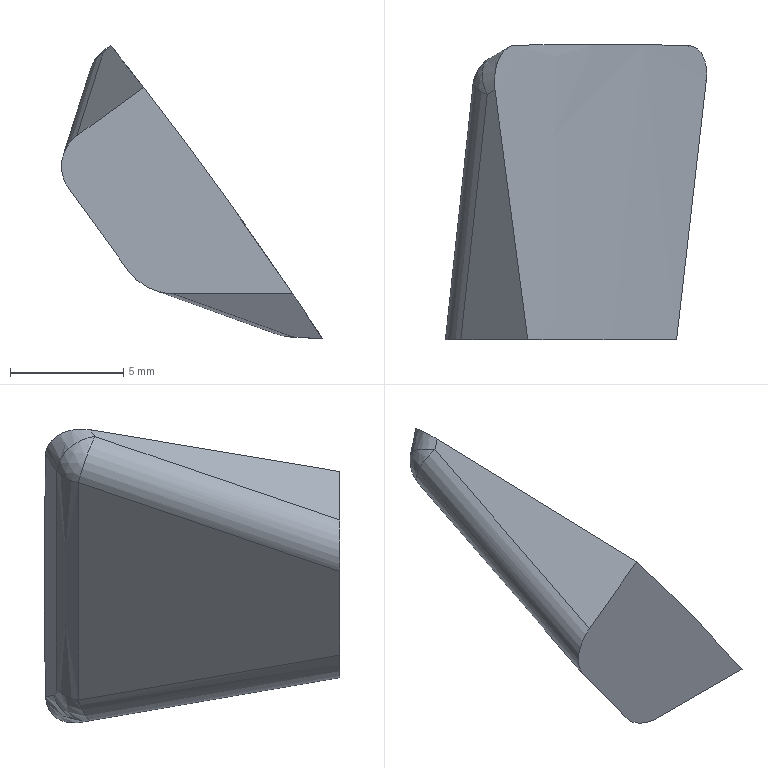Part | STEP file | solid 12 | 1 solid | 13 faces | box 11.557 x 13.074 x 13.001 mm | volume 528.422 mm3 | spline 5 | plane 4 | cylinder 2 | other 1 | sphere 1 | commonest cylinder face diameters 3 x1 4 x1